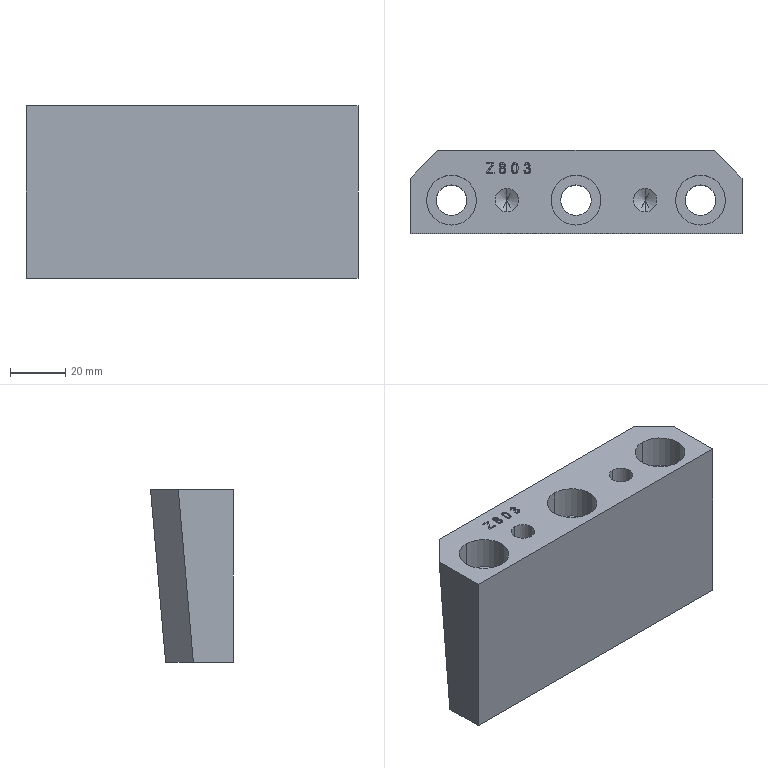Part | Creo | 1 solid | 133 faces | box 120 x 30 x 62.5 mm | volume 171554 mm3 | other 85 | plane 26 | cylinder 18 | cone 4 | commonest cylinder face diameters 11 x6 18 x6 8.5 x4 2.006 x1 54.863 x1